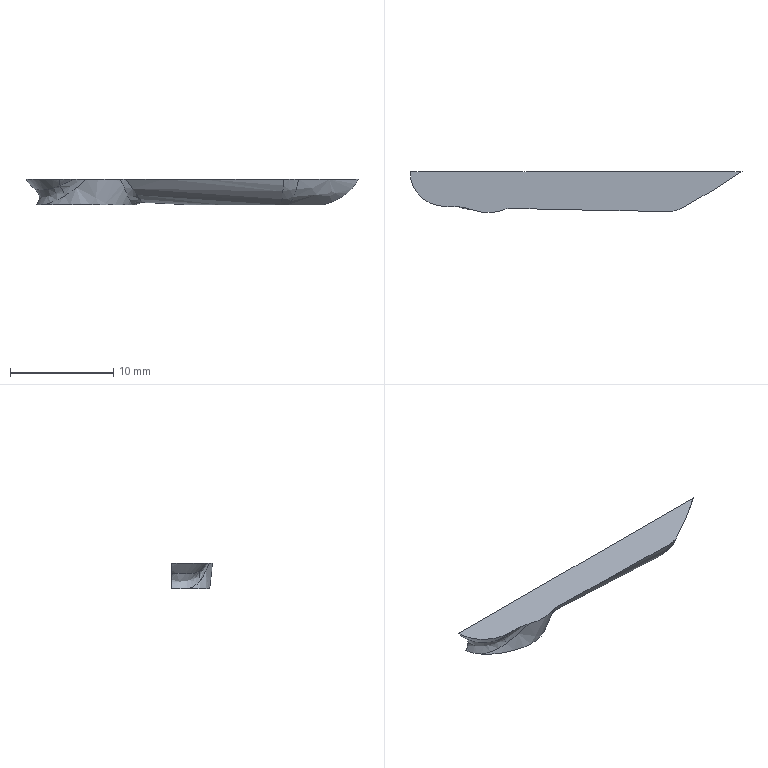Part | STEP file | solid 220 | 1 solid | 13 faces | volume 199.733 mm3 | spline 6 | plane 4 | cylinder 2 | sphere 1 | commonest cylinder face diameters 8 x2